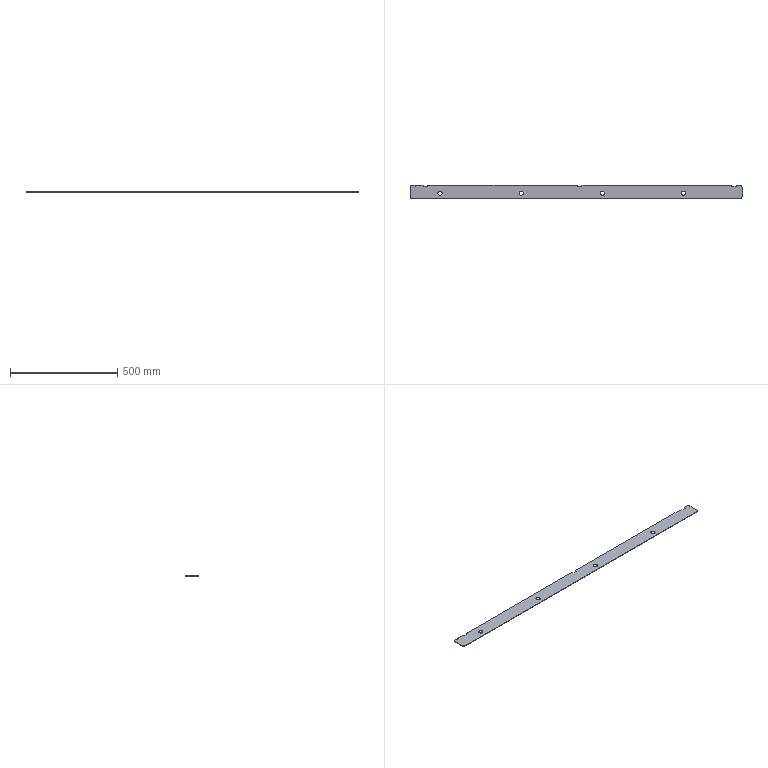Part | SolidWorks | features FlatPattern 1, SMBaseFlange 1, SheetMetal 1 | 1 solid | 34 faces | box 1550 x 65 x 2.3 mm | volume 227708 mm3 | plane 22 | cylinder 12 | commonest cylinder face diameters 20 x12
STEP:
#1=CARTESIAN_POINT('',(1294.,-523.,2.3));
#2=VERTEX_POINT('',#1);
#3=CARTESIAN_POINT('',(1314.,-523.,2.3));
#4=VERTEX_POINT('',#3);
#5=CARTESIAN_POINT('',(1304.,-523.,2.3));
#6=DIRECTION('',(0.,0.,1.));
#7=DIRECTION('',(1.,0.,0.));
#8=AXIS2_PLACEMENT_3D('',#5,#6,#7);
#9=CIRCLE('',#8,10.);
#10=EDGE_CURVE('',#2,#4,#9,.T.);
#11=ORIENTED_EDGE('',*,*,#10,.T.);
#12=CARTESIAN_POINT('',(1314.,-523.,0.));
#13=VERTEX_POINT('',#12);
#14=CARTESIAN_POINT('',(1314.,-523.,2.3));
#15=DIRECTION('',(0.,0.,-1.));
#16=VECTOR('',#15,1000.);
#17=LINE('',#14,#16);
#18=EDGE_CURVE('',#4,#13,#17,.T.);
#19=ORIENTED_EDGE('',*,*,#18,.T.);
#20=CARTESIAN_POINT('',(1294.,-523.,0.));
#21=VERTEX_POINT('',#20);
#22=CARTESIAN_POINT('',(1304.,-523.,0.));
#23=DIRECTION('',(0.,0.,1.));
#24=DIRECTION('',(1.,0.,0.));
#25=AXIS2_PLACEMENT_3D('',#22,#23,#24);
#26=CIRCLE('',#25,10.);
#27=EDGE_CURVE('',#21,#13,#26,.T.);
#28=ORIENTED_EDGE('',*,*,#27,.F.);
#29=CARTESIAN_POINT('',(1294.,-523.,2.3));
#30=DIRECTION('',(0.,0.,-1.));
#31=VECTOR('',#30,1000.);
#32=LINE('',#29,#31);
#33=EDGE_CURVE('',#2,#21,#32,.T.);
#34=ORIENTED_EDGE('',*,*,#33,.F.);
#35=EDGE_LOOP('',(#11,#19,#28,#34));
#36=FACE_OUTER_BOUND('',#35,.T.);
#37=CARTESIAN_POINT('',(1304.,-523.,2.3));
#38=DIRECTION('',(0.,0.,-1.));
#39=DIRECTION('',(-1.,0.,0.));
#40=AXIS2_PLACEMENT_3D('',#37,#38,#39);
#41=CYLINDRICAL_SURFACE('',#40,10.);
#42=ADVANCED_FACE('',(#36),#41,.F.);
#43=CARTESIAN_POINT('',(915.,-523.,2.3));
#44=VERTEX_POINT('',#43);
#45=CARTESIAN_POINT('',(935.,-523.,2.3));
#46=VERTEX_POINT('',#45);
#47=CARTESIAN_POINT('',(925.,-523.,2.3));
#48=DIRECTION('',(0.,0.,1.));
#49=DIRECTION('',(1.,0.,0.));
#50=AXIS2_PLACEMENT_3D('',#47,#48,#49);
#51=CIRCLE('',#50,10.);
#52=EDGE_CURVE('',#44,#46,#51,.T.);
#53=ORIENTED_EDGE('',*,*,#52,.T.);
#54=CARTESIAN_POINT('',(935.,-523.,0.));
#55=VERTEX_POINT('',#54);
#56=CARTESIAN_POINT('',(935.,-523.,2.3));
#57=DIRECTION('',(0.,0.,-1.));
#58=VECTOR('',#57,1000.);
#59=LINE('',#56,#58);
#60=EDGE_CURVE('',#46,#55,#59,.T.);
#61=ORIENTED_EDGE('',*,*,#60,.T.);
#62=CARTESIAN_POINT('',(915.,-523.,0.));
#63=VERTEX_POINT('',#62);
#64=CARTESIAN_POINT('',(925.,-523.,0.));
#65=DIRECTION('',(0.,0.,1.));
#66=DIRECTION('',(1.,0.,0.));
#67=AXIS2_PLACEMENT_3D('',#64,#65,#66);
#68=CIRCLE('',#67,10.);
#69=EDGE_CURVE('',#63,#55,#68,.T.);
#70=ORIENTED_EDGE('',*,*,#69,.F.);
#71=CARTESIAN_POINT('',(915.,-523.,2.3));
#72=DIRECTION('',(0.,0.,-1.));
#73=VECTOR('',#72,1000.);
#74=LINE('',#71,#73);
#75=EDGE_CURVE('',#44,#63,#74,.T.);
#76=ORIENTED_EDGE('',*,*,#75,.F.);
#77=EDGE_LOOP('',(#53,#61,#70,#76));
#78=FACE_OUTER_BOUND('',#77,.T.);
#79=CARTESIAN_POINT('',(925.,-523.,2.3));
#80=DIRECTION('',(0.,0.,-1.));
#81=DIRECTION('',(-1.,0.,0.));
#82=AXIS2_PLACEMENT_3D('',#79,#80,#81);
#83=CYLINDRICAL_SURFACE('',#82,10.);
#84=ADVANCED_FACE('',(#78),#83,.F.);
#85=CARTESIAN_POINT('',(536.,-523.,2.3));
#86=VERTEX_POINT('',#85);
#87=CARTESIAN_POINT('',(556.,-523.,2.3));
#88=VERTEX_POINT('',#87);
#89=CARTESIAN_POINT('',(546.,-523.,2.3));
#90=DIRECTION('',(0.,0.,1.));
#91=DIRECTION('',(1.,0.,0.));
#92=AXIS2_PLACEMENT_3D('',#89,#90,#91);
#93=CIRCLE('',#92,10.);
#94=EDGE_CURVE('',#86,#88,#93,.T.);
#95=ORIENTED_EDGE('',*,*,#94,.T.);
#96=CARTESIAN_POINT('',(556.,-523.,0.));
#97=VERTEX_POINT('',#96);
#98=CARTESIAN_POINT('',(556.,-523.,2.3));
#99=DIRECTION('',(0.,0.,-1.));
#100=VECTOR('',#99,1000.);
#101=LINE('',#98,#100);
#102=EDGE_CURVE('',#88,#97,#101,.T.);
#103=ORIENTED_EDGE('',*,*,#102,.T.);
#104=CARTESIAN_POINT('',(536.,-523.,0.));
#105=VERTEX_POINT('',#104);
#106=CARTESIAN_POINT('',(546.,-523.,0.));
#107=DIRECTION('',(0.,0.,1.));
#108=DIRECTION('',(1.,0.,0.));
#109=AXIS2_PLACEMENT_3D('',#106,#107,#108);
#110=CIRCLE('',#109,10.);
#111=EDGE_CURVE('',#105,#97,#110,.T.);
#112=ORIENTED_EDGE('',*,*,#111,.F.);
#113=CARTESIAN_POINT('',(536.,-523.,2.3));
#114=DIRECTION('',(0.,0.,-1.));
#115=VECTOR('',#114,1000.);
#116=LINE('',#113,#115);
#117=EDGE_CURVE('',#86,#105,#116,.T.);
#118=ORIENTED_EDGE('',*,*,#117,.F.);
#119=EDGE_LOOP('',(#95,#103,#112,#118));
#120=FACE_OUTER_BOUND('',#119,.T.);
#121=CARTESIAN_POINT('',(546.,-523.,2.3));
#122=DIRECTION('',(0.,0.,-1.));
#123=DIRECTION('',(-1.,0.,0.));
#124=AXIS2_PLACEMENT_3D('',#121,#122,#123);
#125=CYLINDRICAL_SURFACE('',#124,10.);
#126=ADVANCED_FACE('',(#120),#125,.F.);
#127=CARTESIAN_POINT('',(157.,-523.,2.3));
#128=VERTEX_POINT('',#127);
#129=CARTESIAN_POINT('',(177.,-523.,2.3));
#130=VERTEX_POINT('',#129);
#131=CARTESIAN_POINT('',(167.,-523.,2.3));
#132=DIRECTION('',(0.,0.,1.));
#133=DIRECTION('',(1.,0.,0.));
#134=AXIS2_PLACEMENT_3D('',#131,#132,#133);
#135=CIRCLE('',#134,10.);
#136=EDGE_CURVE('',#128,#130,#135,.T.);
#137=ORIENTED_EDGE('',*,*,#136,.T.);
#138=CARTESIAN_POINT('',(177.,-523.,0.));
#139=VERTEX_POINT('',#138);
#140=CARTESIAN_POINT('',(177.,-523.,2.3));
#141=DIRECTION('',(0.,0.,-1.));
#142=VECTOR('',#141,1000.);
#143=LINE('',#140,#142);
#144=EDGE_CURVE('',#130,#139,#143,.T.);
#145=ORIENTED_EDGE('',*,*,#144,.T.);
#146=CARTESIAN_POINT('',(157.,-523.,0.));
#147=VERTEX_POINT('',#146);
#148=CARTESIAN_POINT('',(167.,-523.,0.));
#149=DIRECTION('',(0.,0.,1.));
#150=DIRECTION('',(1.,0.,0.));
#151=AXIS2_PLACEMENT_3D('',#148,#149,#150);
#152=CIRCLE('',#151,10.);
#153=EDGE_CURVE('',#147,#139,#152,.T.);
#154=ORIENTED_EDGE('',*,*,#153,.F.);
#155=CARTESIAN_POINT('',(157.,-523.,2.3));
#156=DIRECTION('',(0.,0.,-1.));
#157=VECTOR('',#156,1000.);
#158=LINE('',#155,#157);
#159=EDGE_CURVE('',#128,#147,#158,.T.);
#160=ORIENTED_EDGE('',*,*,#159,.F.);
#161=EDGE_LOOP('',(#137,#145,#154,#160));
#162=FACE_OUTER_BOUND('',#161,.T.);
#163=CARTESIAN_POINT('',(167.,-523.,2.3));
#164=DIRECTION('',(0.,0.,-1.));
#165=DIRECTION('',(-1.,0.,0.));
#166=AXIS2_PLACEMENT_3D('',#163,#164,#165);
#167=CYLINDRICAL_SURFACE('',#166,10.);
#168=ADVANCED_FACE('',(#162),#167,.F.);
#169=CARTESIAN_POINT('',(50.4,-485.,2.3));
#170=VERTEX_POINT('',#169);
#171=CARTESIAN_POINT('',(37.,-485.,2.3));
#172=VERTEX_POINT('',#171);
#173=CARTESIAN_POINT('',(50.4,-485.,2.3));
#174=DIRECTION('',(-1.,0.,0.));
#175=VECTOR('',#174,1000.);
#176=LINE('',#173,#175);
#177=EDGE_CURVE('',#170,#172,#176,.T.);
#178=ORIENTED_EDGE('',*,*,#177,.T.);
#179=CARTESIAN_POINT('',(27.,-495.,2.3));
#180=VERTEX_POINT('',#179);
#181=CARTESIAN_POINT('',(37.,-495.,2.3));
#182=DIRECTION('',(0.,0.,1.));
#183=DIRECTION('',(-1.,0.,0.));
#184=AXIS2_PLACEMENT_3D('',#181,#182,#183);
#185=CIRCLE('',#184,10.);
#186=EDGE_CURVE('',#172,#180,#185,.T.);
#187=ORIENTED_EDGE('',*,*,#186,.T.);
#188=CARTESIAN_POINT('',(27.,-540.,2.3));
#189=VERTEX_POINT('',#188);
#190=CARTESIAN_POINT('',(27.,-540.,2.3));
#191=DIRECTION('',(0.,-1.,0.));
#192=VECTOR('',#191,1000.);
#193=LINE('',#190,#192);
#194=EDGE_CURVE('',#180,#189,#193,.T.);
#195=ORIENTED_EDGE('',*,*,#194,.T.);
#196=CARTESIAN_POINT('',(37.,-550.,2.3));
#197=VERTEX_POINT('',#196);
#198=CARTESIAN_POINT('',(37.,-540.,2.3));
#199=DIRECTION('',(0.,0.,1.));
#200=DIRECTION('',(-1.,0.,0.));
#201=AXIS2_PLACEMENT_3D('',#198,#199,#200);
#202=CIRCLE('',#201,10.);
#203=EDGE_CURVE('',#189,#197,#202,.T.);
#204=ORIENTED_EDGE('',*,*,#203,.T.);
#205=CARTESIAN_POINT('',(1567.,-550.,2.3));
#206=VERTEX_POINT('',#205);
#207=CARTESIAN_POINT('',(37.,-550.,2.3));
#208=DIRECTION('',(1.,0.,0.));
#209=VECTOR('',#208,1000.);
#210=LINE('',#207,#209);
#211=EDGE_CURVE('',#197,#206,#210,.T.);
#212=ORIENTED_EDGE('',*,*,#211,.T.);
#213=CARTESIAN_POINT('',(1577.,-540.,2.3));
#214=VERTEX_POINT('',#213);
#215=CARTESIAN_POINT('',(1567.,-540.,2.3));
#216=DIRECTION('',(0.,0.,1.));
#217=DIRECTION('',(1.,0.,0.));
#218=AXIS2_PLACEMENT_3D('',#215,#216,#217);
#219=CIRCLE('',#218,10.);
#220=EDGE_CURVE('',#206,#214,#219,.T.);
#221=ORIENTED_EDGE('',*,*,#220,.T.);
#222=CARTESIAN_POINT('',(1577.,-495.,2.3));
#223=VERTEX_POINT('',#222);
#224=CARTESIAN_POINT('',(1577.,-540.,2.3));
#225=DIRECTION('',(0.,1.,0.));
#226=VECTOR('',#225,1000.);
#227=LINE('',#224,#226);
#228=EDGE_CURVE('',#214,#223,#227,.T.);
#229=ORIENTED_EDGE('',*,*,#228,.T.);
#230=CARTESIAN_POINT('',(1567.,-485.,2.3));
#231=VERTEX_POINT('',#230);
#232=CARTESIAN_POINT('',(1567.,-495.,2.3));
#233=DIRECTION('',(0.,0.,1.));
#234=DIRECTION('',(1.,0.,0.));
#235=AXIS2_PLACEMENT_3D('',#232,#233,#234);
#236=CIRCLE('',#235,10.);
#237=EDGE_CURVE('',#223,#231,#236,.T.);
#238=ORIENTED_EDGE('',*,*,#237,.T.);
#239=CARTESIAN_POINT('',(1550.,-485.,2.3));
#240=VERTEX_POINT('',#239);
#241=CARTESIAN_POINT('',(1567.,-485.,2.3));
#242=DIRECTION('',(-1.,0.,0.));
#243=VECTOR('',#242,1000.);
#244=LINE('',#241,#243);
#245=EDGE_CURVE('',#231,#240,#244,.T.);
#246=ORIENTED_EDGE('',*,*,#245,.T.);
#247=CARTESIAN_POINT('',(1550.,-491.,2.3));
#248=VERTEX_POINT('',#247);
#249=CARTESIAN_POINT('',(1550.,-485.,2.3));
#250=DIRECTION('',(0.,-1.,0.));
#251=VECTOR('',#250,1000.);
#252=LINE('',#249,#251);
#253=EDGE_CURVE('',#240,#248,#252,.T.);
#254=ORIENTED_EDGE('',*,*,#253,.T.);
#255=CARTESIAN_POINT('',(1528.,-491.,2.3));
#256=VERTEX_POINT('',#255);
#257=CARTESIAN_POINT('',(1550.,-491.,2.3));
#258=DIRECTION('',(-1.,0.,0.));
#259=VECTOR('',#258,1000.);
#260=LINE('',#257,#259);
#261=EDGE_CURVE('',#248,#256,#260,.T.);
#262=ORIENTED_EDGE('',*,*,#261,.T.);
#263=CARTESIAN_POINT('',(1528.,-485.,2.3));
#264=VERTEX_POINT('',#263);
#265=CARTESIAN_POINT('',(1528.,-491.,2.3));
#266=DIRECTION('',(0.,1.,0.));
#267=VECTOR('',#266,1000.);
#268=LINE('',#265,#267);
#269=EDGE_CURVE('',#256,#264,#268,.T.);
#270=ORIENTED_EDGE('',*,*,#269,.T.);
#271=CARTESIAN_POINT('',(830.,-485.,2.3));
#272=VERTEX_POINT('',#271);
#273=CARTESIAN_POINT('',(1528.,-485.,2.3));
#274=DIRECTION('',(-1.,0.,0.));
#275=VECTOR('',#274,1000.);
#276=LINE('',#273,#275);
#277=EDGE_CURVE('',#264,#272,#276,.T.);
#278=ORIENTED_EDGE('',*,*,#277,.T.);
#279=CARTESIAN_POINT('',(830.,-491.,2.3));
#280=VERTEX_POINT('',#279);
#281=CARTESIAN_POINT('',(830.,-485.,2.3));
#282=DIRECTION('',(0.,-1.,0.));
#283=VECTOR('',#282,1000.);
#284=LINE('',#281,#283);
#285=EDGE_CURVE('',#272,#280,#284,.T.);
#286=ORIENTED_EDGE('',*,*,#285,.T.);
#287=CARTESIAN_POINT('',(808.,-491.,2.3));
#288=VERTEX_POINT('',#287);
#289=CARTESIAN_POINT('',(830.,-491.,2.3));
#290=DIRECTION('',(-1.,0.,0.));
#291=VECTOR('',#290,1000.);
#292=LINE('',#289,#291);
#293=EDGE_CURVE('',#280,#288,#292,.T.);
#294=ORIENTED_EDGE('',*,*,#293,.T.);
#295=CARTESIAN_POINT('',(808.,-485.,2.3));
#296=VERTEX_POINT('',#295);
#297=CARTESIAN_POINT('',(808.,-491.,2.3));
#298=DIRECTION('',(0.,1.,0.));
#299=VECTOR('',#298,1000.);
#300=LINE('',#297,#299);
#301=EDGE_CURVE('',#288,#296,#300,.T.);
#302=ORIENTED_EDGE('',*,*,#301,.T.);
#303=CARTESIAN_POINT('',(110.,-485.,2.3));
#304=VERTEX_POINT('',#303);
#305=CARTESIAN_POINT('',(808.,-485.,2.3));
#306=DIRECTION('',(-1.,0.,0.));
#307=VECTOR('',#306,1000.);
#308=LINE('',#305,#307);
#309=EDGE_CURVE('',#296,#304,#308,.T.);
#310=ORIENTED_EDGE('',*,*,#309,.T.);
#311=CARTESIAN_POINT('',(110.,-491.,2.3));
#312=VERTEX_POINT('',#311);
#313=CARTESIAN_POINT('',(110.,-485.,2.3));
#314=DIRECTION('',(0.,-1.,0.));
#315=VECTOR('',#314,1000.);
#316=LINE('',#313,#315);
#317=EDGE_CURVE('',#304,#312,#316,.T.);
#318=ORIENTED_EDGE('',*,*,#317,.T.);
#319=CARTESIAN_POINT('',(88.,-491.,2.3));
#320=VERTEX_POINT('',#319);
#321=CARTESIAN_POINT('',(110.,-491.,2.3));
#322=DIRECTION('',(-1.,0.,0.));
#323=VECTOR('',#322,1000.);
#324=LINE('',#321,#323);
#325=EDGE_CURVE('',#312,#320,#324,.T.);
#326=ORIENTED_EDGE('',*,*,#325,.T.);
#327=CARTESIAN_POINT('',(88.,-485.,2.3));
#328=VERTEX_POINT('',#327);
#329=CARTESIAN_POINT('',(88.,-491.,2.3));
#330=DIRECTION('',(0.,1.,0.));
#331=VECTOR('',#330,1000.);
#332=LINE('',#329,#331);
#333=EDGE_CURVE('',#320,#328,#332,.T.);
#334=ORIENTED_EDGE('',*,*,#333,.T.);
#335=CARTESIAN_POINT('',(52.,-485.,2.3));
#336=VERTEX_POINT('',#335);
#337=CARTESIAN_POINT('',(88.,-485.,2.3));
#338=DIRECTION('',(-1.,0.,0.));
#339=VECTOR('',#338,1000.);
#340=LINE('',#337,#339);
#341=EDGE_CURVE('',#328,#336,#340,.T.);
#342=ORIENTED_EDGE('',*,*,#341,.T.);
#343=CARTESIAN_POINT('',(52.,-490.,2.3));
#344=VERTEX_POINT('',#343);
#345=CARTESIAN_POINT('',(52.,-490.,2.3));
#346=DIRECTION('',(0.,-1.,0.));
#347=VECTOR('',#346,1000.);
#348=LINE('',#345,#347);
#349=EDGE_CURVE('',#336,#344,#348,.T.);
#350=ORIENTED_EDGE('',*,*,#349,.T.);
#351=CARTESIAN_POINT('',(50.4,-490.,2.3));
#352=VERTEX_POINT('',#351);
#353=CARTESIAN_POINT('',(52.,-490.,2.3));
#354=DIRECTION('',(-1.,0.,0.));
#355=VECTOR('',#354,1000.);
#356=LINE('',#353,#355);
#357=EDGE_CURVE('',#344,#352,#356,.T.);
#358=ORIENTED_EDGE('',*,*,#357,.T.);
#359=CARTESIAN_POINT('',(50.4,-490.,2.3));
#360=DIRECTION('',(0.,1.,0.));
#361=VECTOR('',#360,1000.);
#362=LINE('',#359,#361);
#363=EDGE_CURVE('',#352,#170,#362,.T.);
#364=ORIENTED_EDGE('',*,*,#363,.T.);
#365=EDGE_LOOP('',(#178,#187,#195,#204,#212,#221,#229,#238,#246,#254,#262,#270,#278,#286,#294,#302,#310,#318,#326,#334,#342,#350,#358,#364));
#366=FACE_OUTER_BOUND('',#365,.T.);
#367=ORIENTED_EDGE('',*,*,#136,.F.);
#368=CARTESIAN_POINT('',(167.,-523.,2.3));
#369=DIRECTION('',(0.,0.,1.));
#370=DIRECTION('',(1.,0.,0.));
#371=AXIS2_PLACEMENT_3D('',#368,#369,#370);
#372=CIRCLE('',#371,10.);
#373=EDGE_CURVE('',#130,#128,#372,.T.);
#374=ORIENTED_EDGE('',*,*,#373,.F.);
#375=EDGE_LOOP('',(#367,#374));
#376=FACE_BOUND('',#375,.T.);
#377=ORIENTED_EDGE('',*,*,#94,.F.);
#378=CARTESIAN_POINT('',(546.,-523.,2.3));
#379=DIRECTION('',(0.,0.,1.));
#380=DIRECTION('',(1.,0.,0.));
#381=AXIS2_PLACEMENT_3D('',#378,#379,#380);
#382=CIRCLE('',#381,10.);
#383=EDGE_CURVE('',#88,#86,#382,.T.);
#384=ORIENTED_EDGE('',*,*,#383,.F.);
#385=EDGE_LOOP('',(#377,#384));
#386=FACE_BOUND('',#385,.T.);
#387=ORIENTED_EDGE('',*,*,#52,.F.);
#388=CARTESIAN_POINT('',(925.,-523.,2.3));
#389=DIRECTION('',(0.,0.,1.));
#390=DIRECTION('',(1.,0.,0.));
#391=AXIS2_PLACEMENT_3D('',#388,#389,#390);
#392=CIRCLE('',#391,10.);
#393=EDGE_CURVE('',#46,#44,#392,.T.);
#394=ORIENTED_EDGE('',*,*,#393,.F.);
#395=EDGE_LOOP('',(#387,#394));
#396=FACE_BOUND('',#395,.T.);
#397=ORIENTED_EDGE('',*,*,#10,.F.);
#398=CARTESIAN_POINT('',(1304.,-523.,2.3));
#399=DIRECTION('',(0.,0.,1.));
#400=DIRECTION('',(1.,0.,0.));
#401=AXIS2_PLACEMENT_3D('',#398,#399,#400);
#402=CIRCLE('',#401,10.);
#403=EDGE_CURVE('',#4,#2,#402,.T.);
#404=ORIENTED_EDGE('',*,*,#403,.F.);
#405=EDGE_LOOP('',(#397,#404));
#406=FACE_BOUND('',#405,.T.);
#407=CARTESIAN_POINT('',(37.,-495.,2.3));
#408=DIRECTION('',(0.,0.,-1.));
#409=DIRECTION('',(-1.,0.,0.));
#410=AXIS2_PLACEMENT_3D('',#407,#408,#409);
#411=PLANE('',#410);
#412=ADVANCED_FACE('',(#366,#376,#386,#396,#406),#411,.F.);
#413=ORIENTED_EDGE('',*,*,#69,.T.);
#414=CARTESIAN_POINT('',(925.,-523.,0.));
#415=DIRECTION('',(0.,0.,1.));
#416=DIRECTION('',(1.,0.,0.));
#417=AXIS2_PLACEMENT_3D('',#414,#415,#416);
#418=CIRCLE('',#417,10.);
#419=EDGE_CURVE('',#55,#63,#418,.T.);
#420=ORIENTED_EDGE('',*,*,#419,.T.);
#421=EDGE_LOOP('',(#413,#420));
#422=FACE_BOUND('',#421,.T.);
#423=ORIENTED_EDGE('',*,*,#153,.T.);
#424=CARTESIAN_POINT('',(167.,-523.,0.));
#425=DIRECTION('',(0.,0.,1.));
#426=DIRECTION('',(1.,0.,0.));
#427=AXIS2_PLACEMENT_3D('',#424,#425,#426);
#428=CIRCLE('',#427,10.);
#429=EDGE_CURVE('',#139,#147,#428,.T.);
#430=ORIENTED_EDGE('',*,*,#429,.T.);
#431=EDGE_LOOP('',(#423,#430));
#432=FACE_BOUND('',#431,.T.);
#433=CARTESIAN_POINT('',(50.4,-485.,0.));
#434=VERTEX_POINT('',#433);
#435=CARTESIAN_POINT('',(37.,-485.,0.));
#436=VERTEX_POINT('',#435);
#437=CARTESIAN_POINT('',(50.4,-485.,0.));
#438=DIRECTION('',(-1.,0.,0.));
#439=VECTOR('',#438,1000.);
#440=LINE('',#437,#439);
#441=EDGE_CURVE('',#434,#436,#440,.T.);
#442=ORIENTED_EDGE('',*,*,#441,.F.);
#443=CARTESIAN_POINT('',(50.4,-490.,0.));
#444=VERTEX_POINT('',#443);
#445=CARTESIAN_POINT('',(50.4,-490.,0.));
#446=DIRECTION('',(0.,1.,0.));
#447=VECTOR('',#446,1000.);
#448=LINE('',#445,#447);
#449=EDGE_CURVE('',#444,#434,#448,.T.);
#450=ORIENTED_EDGE('',*,*,#449,.F.);
#451=CARTESIAN_POINT('',(52.,-490.,0.));
#452=VERTEX_POINT('',#451);
#453=CARTESIAN_POINT('',(52.,-490.,0.));
#454=DIRECTION('',(-1.,0.,0.));
#455=VECTOR('',#454,1000.);
#456=LINE('',#453,#455);
#457=EDGE_CURVE('',#452,#444,#456,.T.);
#458=ORIENTED_EDGE('',*,*,#457,.F.);
#459=CARTESIAN_POINT('',(52.,-485.,0.));
#460=VERTEX_POINT('',#459);
#461=CARTESIAN_POINT('',(52.,-490.,0.));
#462=DIRECTION('',(0.,-1.,0.));
#463=VECTOR('',#462,1000.);
#464=LINE('',#461,#463);
#465=EDGE_CURVE('',#460,#452,#464,.T.);
#466=ORIENTED_EDGE('',*,*,#465,.F.);
#467=CARTESIAN_POINT('',(88.,-485.,0.));
#468=VERTEX_POINT('',#467);
#469=CARTESIAN_POINT('',(88.,-485.,0.));
#470=DIRECTION('',(-1.,0.,0.));
#471=VECTOR('',#470,1000.);
#472=LINE('',#469,#471);
#473=EDGE_CURVE('',#468,#460,#472,.T.);
#474=ORIENTED_EDGE('',*,*,#473,.F.);
#475=CARTESIAN_POINT('',(88.,-491.,0.));
#476=VERTEX_POINT('',#475);
#477=CARTESIAN_POINT('',(88.,-491.,0.));
#478=DIRECTION('',(0.,1.,0.));
#479=VECTOR('',#478,1000.);
#480=LINE('',#477,#479);
#481=EDGE_CURVE('',#476,#468,#480,.T.);
#482=ORIENTED_EDGE('',*,*,#481,.F.);
#483=CARTESIAN_POINT('',(110.,-491.,0.));
#484=VERTEX_POINT('',#483);
#485=CARTESIAN_POINT('',(110.,-491.,0.));
#486=DIRECTION('',(-1.,0.,0.));
#487=VECTOR('',#486,1000.);
#488=LINE('',#485,#487);
#489=EDGE_CURVE('',#484,#476,#488,.T.);
#490=ORIENTED_EDGE('',*,*,#489,.F.);
#491=CARTESIAN_POINT('',(110.,-485.,0.));
#492=VERTEX_POINT('',#491);
#493=CARTESIAN_POINT('',(110.,-485.,0.));
#494=DIRECTION('',(0.,-1.,0.));
#495=VECTOR('',#494,1000.);
#496=LINE('',#493,#495);
#497=EDGE_CURVE('',#492,#484,#496,.T.);
#498=ORIENTED_EDGE('',*,*,#497,.F.);
#499=CARTESIAN_POINT('',(808.,-485.,0.));
#500=VERTEX_POINT('',#499);
#501=CARTESIAN_POINT('',(808.,-485.,0.));
#502=DIRECTION('',(-1.,0.,0.));
#503=VECTOR('',#502,1000.);
#504=LINE('',#501,#503);
#505=EDGE_CURVE('',#500,#492,#504,.T.);
#506=ORIENTED_EDGE('',*,*,#505,.F.);
#507=CARTESIAN_POINT('',(808.,-491.,0.));
#508=VERTEX_POINT('',#507);
#509=CARTESIAN_POINT('',(808.,-491.,0.));
#510=DIRECTION('',(0.,1.,0.));
#511=VECTOR('',#510,1000.);
#512=LINE('',#509,#511);
#513=EDGE_CURVE('',#508,#500,#512,.T.);
#514=ORIENTED_EDGE('',*,*,#513,.F.);
#515=CARTESIAN_POINT('',(830.,-491.,0.));
#516=VERTEX_POINT('',#515);
#517=CARTESIAN_POINT('',(830.,-491.,0.));
#518=DIRECTION('',(-1.,0.,0.));
#519=VECTOR('',#518,1000.);
#520=LINE('',#517,#519);
#521=EDGE_CURVE('',#516,#508,#520,.T.);
#522=ORIENTED_EDGE('',*,*,#521,.F.);
#523=CARTESIAN_POINT('',(830.,-485.,0.));
#524=VERTEX_POINT('',#523);
#525=CARTESIAN_POINT('',(830.,-485.,0.));
#526=DIRECTION('',(0.,-1.,0.));
#527=VECTOR('',#526,1000.);
#528=LINE('',#525,#527);
#529=EDGE_CURVE('',#524,#516,#528,.T.);
#530=ORIENTED_EDGE('',*,*,#529,.F.);
#531=CARTESIAN_POINT('',(1528.,-485.,0.));
#532=VERTEX_POINT('',#531);
#533=CARTESIAN_POINT('',(1528.,-485.,0.));
#534=DIRECTION('',(-1.,0.,0.));
#535=VECTOR('',#534,1000.);
#536=LINE('',#533,#535);
#537=EDGE_CURVE('',#532,#524,#536,.T.);
#538=ORIENTED_EDGE('',*,*,#537,.F.);
#539=CARTESIAN_POINT('',(1528.,-491.,0.));
#540=VERTEX_POINT('',#539);
#541=CARTESIAN_POINT('',(1528.,-491.,0.));
#542=DIRECTION('',(0.,1.,0.));
#543=VECTOR('',#542,1000.);
#544=LINE('',#541,#543);
#545=EDGE_CURVE('',#540,#532,#544,.T.);
#546=ORIENTED_EDGE('',*,*,#545,.F.);
#547=CARTESIAN_POINT('',(1550.,-491.,0.));
#548=VERTEX_POINT('',#547);
#549=CARTESIAN_POINT('',(1550.,-491.,0.));
#550=DIRECTION('',(-1.,0.,0.));
#551=VECTOR('',#550,1000.);
#552=LINE('',#549,#551);
#553=EDGE_CURVE('',#548,#540,#552,.T.);
#554=ORIENTED_EDGE('',*,*,#553,.F.);
#555=CARTESIAN_POINT('',(1550.,-485.,0.));
#556=VERTEX_POINT('',#555);
#557=CARTESIAN_POINT('',(1550.,-485.,0.));
#558=DIRECTION('',(0.,-1.,0.));
#559=VECTOR('',#558,1000.);
#560=LINE('',#557,#559);
#561=EDGE_CURVE('',#556,#548,#560,.T.);
#562=ORIENTED_EDGE('',*,*,#561,.F.);
#563=CARTESIAN_POINT('',(1567.,-485.,0.));
#564=VERTEX_POINT('',#563);
#565=CARTESIAN_POINT('',(1567.,-485.,0.));
#566=DIRECTION('',(-1.,0.,0.));
#567=VECTOR('',#566,1000.);
#568=LINE('',#565,#567);
#569=EDGE_CURVE('',#564,#556,#568,.T.);
#570=ORIENTED_EDGE('',*,*,#569,.F.);
#571=CARTESIAN_POINT('',(1577.,-495.,0.));
#572=VERTEX_POINT('',#571);
#573=CARTESIAN_POINT('',(1567.,-495.,0.));
#574=DIRECTION('',(0.,0.,1.));
#575=DIRECTION('',(1.,0.,0.));
#576=AXIS2_PLACEMENT_3D('',#573,#574,#575);
#577=CIRCLE('',#576,10.);
#578=EDGE_CURVE('',#572,#564,#577,.T.);
#579=ORIENTED_EDGE('',*,*,#578,.F.);
#580=CARTESIAN_POINT('',(1577.,-540.,0.));
#581=VERTEX_POINT('',#580);
#582=CARTESIAN_POINT('',(1577.,-540.,0.));
#583=DIRECTION('',(0.,1.,0.));
#584=VECTOR('',#583,1000.);
#585=LINE('',#582,#584);
#586=EDGE_CURVE('',#581,#572,#585,.T.);
#587=ORIENTED_EDGE('',*,*,#586,.F.);
#588=CARTESIAN_POINT('',(1567.,-550.,0.));
#589=VERTEX_POINT('',#588);
#590=CARTESIAN_POINT('',(1567.,-540.,0.));
#591=DIRECTION('',(0.,0.,1.));
#592=DIRECTION('',(1.,0.,0.));
#593=AXIS2_PLACEMENT_3D('',#590,#591,#592);
#594=CIRCLE('',#593,10.);
#595=EDGE_CURVE('',#589,#581,#594,.T.);
#596=ORIENTED_EDGE('',*,*,#595,.F.);
#597=CARTESIAN_POINT('',(37.,-550.,0.));
#598=VERTEX_POINT('',#597);
#599=CARTESIAN_POINT('',(37.,-550.,0.));
#600=DIRECTION('',(1.,0.,0.));
#601=VECTOR('',#600,1000.);
#602=LINE('',#599,#601);
#603=EDGE_CURVE('',#598,#589,#602,.T.);
#604=ORIENTED_EDGE('',*,*,#603,.F.);
#605=CARTESIAN_POINT('',(27.,-540.,0.));
#606=VERTEX_POINT('',#605);
#607=CARTESIAN_POINT('',(37.,-540.,0.));
#608=DIRECTION('',(0.,0.,1.));
#609=DIRECTION('',(-1.,0.,0.));
#610=AXIS2_PLACEMENT_3D('',#607,#608,#609);
#611=CIRCLE('',#610,10.);
#612=EDGE_CURVE('',#606,#598,#611,.T.);
#613=ORIENTED_EDGE('',*,*,#612,.F.);
#614=CARTESIAN_POINT('',(27.,-495.,0.));
#615=VERTEX_POINT('',#614);
#616=CARTESIAN_POINT('',(27.,-540.,0.));
#617=DIRECTION('',(0.,-1.,0.));
#618=VECTOR('',#617,1000.);
#619=LINE('',#616,#618);
#620=EDGE_CURVE('',#615,#606,#619,.T.);
#621=ORIENTED_EDGE('',*,*,#620,.F.);
#622=CARTESIAN_POINT('',(37.,-495.,0.));
#623=DIRECTION('',(0.,0.,1.));
#624=DIRECTION('',(-1.,0.,0.));
#625=AXIS2_PLACEMENT_3D('',#622,#623,#624);
#626=CIRCLE('',#625,10.);
#627=EDGE_CURVE('',#436,#615,#626,.T.);
#628=ORIENTED_EDGE('',*,*,#627,.F.);
#629=EDGE_LOOP('',(#442,#450,#458,#466,#474,#482,#490,#498,#506,#514,#522,#530,#538,#546,#554,#562,#570,#579,#587,#596,#604,#613,#621,#628));
#630=FACE_OUTER_BOUND('',#629,.T.);
#631=ORIENTED_EDGE('',*,*,#111,.T.);
#632=CARTESIAN_POINT('',(546.,-523.,0.));
#633=DIRECTION('',(0.,0.,1.));
#634=DIRECTION('',(1.,0.,0.));
#635=AXIS2_PLACEMENT_3D('',#632,#633,#634);
#636=CIRCLE('',#635,10.);
#637=EDGE_CURVE('',#97,#105,#636,.T.);
#638=ORIENTED_EDGE('',*,*,#637,.T.);
#639=EDGE_LOOP('',(#631,#638));
#640=FACE_BOUND('',#639,.T.);
#641=ORIENTED_EDGE('',*,*,#27,.T.);
#642=CARTESIAN_POINT('',(1304.,-523.,0.));
#643=DIRECTION('',(0.,0.,1.));
#644=DIRECTION('',(1.,0.,0.));
#645=AXIS2_PLACEMENT_3D('',#642,#643,#644);
#646=CIRCLE('',#645,10.);
#647=EDGE_CURVE('',#13,#21,#646,.T.);
#648=ORIENTED_EDGE('',*,*,#647,.T.);
#649=EDGE_LOOP('',(#641,#648));
#650=FACE_BOUND('',#649,.T.);
#651=CARTESIAN_POINT('',(37.,-495.,0.));
#652=DIRECTION('',(0.,0.,-1.));
#653=DIRECTION('',(-1.,0.,0.));
#654=AXIS2_PLACEMENT_3D('',#651,#652,#653);
#655=PLANE('',#654);
#656=ADVANCED_FACE('',(#422,#432,#630,#640,#650),#655,.T.);
#657=ORIENTED_EDGE('',*,*,#441,.T.);
#658=CARTESIAN_POINT('',(37.,-485.,2.3));
#659=DIRECTION('',(0.,0.,-1.));
#660=VECTOR('',#659,1000.);
#661=LINE('',#658,#660);
#662=EDGE_CURVE('',#172,#436,#661,.T.);
#663=ORIENTED_EDGE('',*,*,#662,.F.);
#664=ORIENTED_EDGE('',*,*,#177,.F.);
#665=CARTESIAN_POINT('',(50.4,-485.,2.3));
#666=DIRECTION('',(0.,0.,-1.));
#667=VECTOR('',#666,1000.);
#668=LINE('',#665,#667);
#669=EDGE_CURVE('',#170,#434,#668,.T.);
#670=ORIENTED_EDGE('',*,*,#669,.T.);
#671=EDGE_LOOP('',(#657,#663,#664,#670));
#672=FACE_OUTER_BOUND('',#671,.T.);
#673=CARTESIAN_POINT('',(50.4,-485.,2.3));
#674=DIRECTION('',(0.,-1.,0.));
#675=DIRECTION('',(0.,0.,-1.));
#676=AXIS2_PLACEMENT_3D('',#673,#674,#675);
#677=PLANE('',#676);
#678=ADVANCED_FACE('',(#672),#677,.F.);
#679=ORIENTED_EDGE('',*,*,#627,.T.);
#680=CARTESIAN_POINT('',(27.,-495.,2.3));
#681=DIRECTION('',(0.,0.,-1.));
#682=VECTOR('',#681,1000.);
#683=LINE('',#680,#682);
#684=EDGE_CURVE('',#180,#615,#683,.T.);
#685=ORIENTED_EDGE('',*,*,#684,.F.);
#686=ORIENTED_EDGE('',*,*,#186,.F.);
#687=ORIENTED_EDGE('',*,*,#662,.T.);
#688=EDGE_LOOP('',(#679,#685,#686,#687));
#689=FACE_OUTER_BOUND('',#688,.T.);
#690=CARTESIAN_POINT('',(37.,-495.,2.3));
#691=DIRECTION('',(0.,0.,-1.));
#692=DIRECTION('',(-1.,0.,0.));
#693=AXIS2_PLACEMENT_3D('',#690,#691,#692);
#694=CYLINDRICAL_SURFACE('',#693,10.);
#695=ADVANCED_FACE('',(#689),#694,.T.);
#696=ORIENTED_EDGE('',*,*,#620,.T.);
#697=CARTESIAN_POINT('',(27.,-540.,2.3));
#698=DIRECTION('',(0.,0.,-1.));
#699=VECTOR('',#698,1000.);
#700=LINE('',#697,#699);
#701=EDGE_CURVE('',#189,#606,#700,.T.);
#702=ORIENTED_EDGE('',*,*,#701,.F.);
#703=ORIENTED_EDGE('',*,*,#194,.F.);
#704=ORIENTED_EDGE('',*,*,#684,.T.);
#705=EDGE_LOOP('',(#696,#702,#703,#704));
#706=FACE_OUTER_BOUND('',#705,.T.);
#707=CARTESIAN_POINT('',(27.,-540.,2.3));
#708=DIRECTION('',(1.,0.,0.));
#709=DIRECTION('',(0.,0.,-1.));
#710=AXIS2_PLACEMENT_3D('',#707,#708,#709);
#711=PLANE('',#710);
#712=ADVANCED_FACE('',(#706),#711,.F.);
#713=ORIENTED_EDGE('',*,*,#612,.T.);
#714=CARTESIAN_POINT('',(37.,-550.,2.3));
#715=DIRECTION('',(0.,0.,-1.));
#716=VECTOR('',#715,1000.);
#717=LINE('',#714,#716);
#718=EDGE_CURVE('',#197,#598,#717,.T.);
#719=ORIENTED_EDGE('',*,*,#718,.F.);
#720=ORIENTED_EDGE('',*,*,#203,.F.);
#721=ORIENTED_EDGE('',*,*,#701,.T.);
#722=EDGE_LOOP('',(#713,#719,#720,#721));
#723=FACE_OUTER_BOUND('',#722,.T.);
#724=CARTESIAN_POINT('',(37.,-540.,2.3));
#725=DIRECTION('',(0.,0.,-1.));
#726=DIRECTION('',(-1.,0.,0.));
#727=AXIS2_PLACEMENT_3D('',#724,#725,#726);
#728=CYLINDRICAL_SURFACE('',#727,10.);
#729=ADVANCED_FACE('',(#723),#728,.T.);
#730=ORIENTED_EDGE('',*,*,#603,.T.);
#731=CARTESIAN_POINT('',(1567.,-550.,2.3));
#732=DIRECTION('',(0.,0.,-1.));
#733=VECTOR('',#732,1000.);
#734=LINE('',#731,#733);
#735=EDGE_CURVE('',#206,#589,#734,.T.);
#736=ORIENTED_EDGE('',*,*,#735,.F.);
#737=ORIENTED_EDGE('',*,*,#211,.F.);
#738=ORIENTED_EDGE('',*,*,#718,.T.);
#739=EDGE_LOOP('',(#730,#736,#737,#738));
#740=FACE_OUTER_BOUND('',#739,.T.);
#741=CARTESIAN_POINT('',(37.,-550.,2.3));
#742=DIRECTION('',(0.,1.,0.));
#743=DIRECTION('',(0.,0.,1.));
#744=AXIS2_PLACEMENT_3D('',#741,#742,#743);
#745=PLANE('',#744);
#746=ADVANCED_FACE('',(#740),#745,.F.);
#747=ORIENTED_EDGE('',*,*,#595,.T.);
#748=CARTESIAN_POINT('',(1577.,-540.,2.3));
#749=DIRECTION('',(0.,0.,-1.));
#750=VECTOR('',#749,1000.);
#751=LINE('',#748,#750);
#752=EDGE_CURVE('',#214,#581,#751,.T.);
#753=ORIENTED_EDGE('',*,*,#752,.F.);
#754=ORIENTED_EDGE('',*,*,#220,.F.);
#755=ORIENTED_EDGE('',*,*,#735,.T.);
#756=EDGE_LOOP('',(#747,#753,#754,#755));
#757=FACE_OUTER_BOUND('',#756,.T.);
#758=CARTESIAN_POINT('',(1567.,-540.,2.3));
#759=DIRECTION('',(0.,0.,-1.));
#760=DIRECTION('',(-1.,0.,0.));
#761=AXIS2_PLACEMENT_3D('',#758,#759,#760);
#762=CYLINDRICAL_SURFACE('',#761,10.);
#763=ADVANCED_FACE('',(#757),#762,.T.);
#764=ORIENTED_EDGE('',*,*,#586,.T.);
#765=CARTESIAN_POINT('',(1577.,-495.,2.3));
#766=DIRECTION('',(0.,0.,-1.));
#767=VECTOR('',#766,1000.);
#768=LINE('',#765,#767);
#769=EDGE_CURVE('',#223,#572,#768,.T.);
#770=ORIENTED_EDGE('',*,*,#769,.F.);
#771=ORIENTED_EDGE('',*,*,#228,.F.);
#772=ORIENTED_EDGE('',*,*,#752,.T.);
#773=EDGE_LOOP('',(#764,#770,#771,#772));
#774=FACE_OUTER_BOUND('',#773,.T.);
#775=CARTESIAN_POINT('',(1577.,-540.,2.3));
#776=DIRECTION('',(-1.,0.,0.));
#777=DIRECTION('',(0.,0.,1.));
#778=AXIS2_PLACEMENT_3D('',#775,#776,#777);
#779=PLANE('',#778);
#780=ADVANCED_FACE('',(#774),#779,.F.);
#781=ORIENTED_EDGE('',*,*,#578,.T.);
#782=CARTESIAN_POINT('',(1567.,-485.,2.3));
#783=DIRECTION('',(0.,0.,-1.));
#784=VECTOR('',#783,1000.);
#785=LINE('',#782,#784);
#786=EDGE_CURVE('',#231,#564,#785,.T.);
#787=ORIENTED_EDGE('',*,*,#786,.F.);
#788=ORIENTED_EDGE('',*,*,#237,.F.);
#789=ORIENTED_EDGE('',*,*,#769,.T.);
#790=EDGE_LOOP('',(#781,#787,#788,#789));
#791=FACE_OUTER_BOUND('',#790,.T.);
#792=CARTESIAN_POINT('',(1567.,-495.,2.3));
#793=DIRECTION('',(0.,0.,-1.));
#794=DIRECTION('',(-1.,0.,0.));
#795=AXIS2_PLACEMENT_3D('',#792,#793,#794);
#796=CYLINDRICAL_SURFACE('',#795,10.);
#797=ADVANCED_FACE('',(#791),#796,.T.);
#798=ORIENTED_EDGE('',*,*,#569,.T.);
#799=CARTESIAN_POINT('',(1550.,-485.,2.3));
#800=DIRECTION('',(0.,0.,-1.));
#801=VECTOR('',#800,1000.);
#802=LINE('',#799,#801);
#803=EDGE_CURVE('',#240,#556,#802,.T.);
#804=ORIENTED_EDGE('',*,*,#803,.F.);
#805=ORIENTED_EDGE('',*,*,#245,.F.);
#806=ORIENTED_EDGE('',*,*,#786,.T.);
#807=EDGE_LOOP('',(#798,#804,#805,#806));
#808=FACE_OUTER_BOUND('',#807,.T.);
#809=CARTESIAN_POINT('',(1567.,-485.,2.3));
#810=DIRECTION('',(0.,-1.,0.));
#811=DIRECTION('',(0.,0.,-1.));
#812=AXIS2_PLACEMENT_3D('',#809,#810,#811);
#813=PLANE('',#812);
#814=ADVANCED_FACE('',(#808),#813,.F.);
#815=ORIENTED_EDGE('',*,*,#561,.T.);
#816=CARTESIAN_POINT('',(1550.,-491.,2.3));
#817=DIRECTION('',(0.,0.,-1.));
#818=VECTOR('',#817,1000.);
#819=LINE('',#816,#818);
#820=EDGE_CURVE('',#248,#548,#819,.T.);
#821=ORIENTED_EDGE('',*,*,#820,.F.);
#822=ORIENTED_EDGE('',*,*,#253,.F.);
#823=ORIENTED_EDGE('',*,*,#803,.T.);
#824=EDGE_LOOP('',(#815,#821,#822,#823));
#825=FACE_OUTER_BOUND('',#824,.T.);
#826=CARTESIAN_POINT('',(1550.,-485.,2.3));
#827=DIRECTION('',(1.,0.,0.));
#828=DIRECTION('',(0.,0.,-1.));
#829=AXIS2_PLACEMENT_3D('',#826,#827,#828);
#830=PLANE('',#829);
#831=ADVANCED_FACE('',(#825),#830,.F.);
#832=ORIENTED_EDGE('',*,*,#553,.T.);
#833=CARTESIAN_POINT('',(1528.,-491.,2.3));
#834=DIRECTION('',(0.,0.,-1.));
#835=VECTOR('',#834,1000.);
#836=LINE('',#833,#835);
#837=EDGE_CURVE('',#256,#540,#836,.T.);
#838=ORIENTED_EDGE('',*,*,#837,.F.);
#839=ORIENTED_EDGE('',*,*,#261,.F.);
#840=ORIENTED_EDGE('',*,*,#820,.T.);
#841=EDGE_LOOP('',(#832,#838,#839,#840));
#842=FACE_OUTER_BOUND('',#841,.T.);
#843=CARTESIAN_POINT('',(1550.,-491.,2.3));
#844=DIRECTION('',(0.,-1.,0.));
#845=DIRECTION('',(0.,0.,-1.));
#846=AXIS2_PLACEMENT_3D('',#843,#844,#845);
#847=PLANE('',#846);
#848=ADVANCED_FACE('',(#842),#847,.F.);
#849=ORIENTED_EDGE('',*,*,#545,.T.);
#850=CARTESIAN_POINT('',(1528.,-485.,2.3));
#851=DIRECTION('',(0.,0.,-1.));
#852=VECTOR('',#851,1000.);
#853=LINE('',#850,#852);
#854=EDGE_CURVE('',#264,#532,#853,.T.);
#855=ORIENTED_EDGE('',*,*,#854,.F.);
#856=ORIENTED_EDGE('',*,*,#269,.F.);
#857=ORIENTED_EDGE('',*,*,#837,.T.);
#858=EDGE_LOOP('',(#849,#855,#856,#857));
#859=FACE_OUTER_BOUND('',#858,.T.);
#860=CARTESIAN_POINT('',(1528.,-491.,2.3));
#861=DIRECTION('',(-1.,0.,0.));
#862=DIRECTION('',(0.,0.,1.));
#863=AXIS2_PLACEMENT_3D('',#860,#861,#862);
#864=PLANE('',#863);
#865=ADVANCED_FACE('',(#859),#864,.F.);
#866=ORIENTED_EDGE('',*,*,#537,.T.);
#867=CARTESIAN_POINT('',(830.,-485.,2.3));
#868=DIRECTION('',(0.,0.,-1.));
#869=VECTOR('',#868,1000.);
#870=LINE('',#867,#869);
#871=EDGE_CURVE('',#272,#524,#870,.T.);
#872=ORIENTED_EDGE('',*,*,#871,.F.);
#873=ORIENTED_EDGE('',*,*,#277,.F.);
#874=ORIENTED_EDGE('',*,*,#854,.T.);
#875=EDGE_LOOP('',(#866,#872,#873,#874));
#876=FACE_OUTER_BOUND('',#875,.T.);
#877=CARTESIAN_POINT('',(1528.,-485.,2.3));
#878=DIRECTION('',(0.,-1.,0.));
#879=DIRECTION('',(1.,0.,0.));
#880=AXIS2_PLACEMENT_3D('',#877,#878,#879);
#881=PLANE('',#880);
#882=ADVANCED_FACE('',(#876),#881,.F.);
#883=ORIENTED_EDGE('',*,*,#529,.T.);
#884=CARTESIAN_POINT('',(830.,-491.,2.3));
#885=DIRECTION('',(0.,0.,-1.));
#886=VECTOR('',#885,1000.);
#887=LINE('',#884,#886);
#888=EDGE_CURVE('',#280,#516,#887,.T.);
#889=ORIENTED_EDGE('',*,*,#888,.F.);
#890=ORIENTED_EDGE('',*,*,#285,.F.);
#891=ORIENTED_EDGE('',*,*,#871,.T.);
#892=EDGE_LOOP('',(#883,#889,#890,#891));
#893=FACE_OUTER_BOUND('',#892,.T.);
#894=CARTESIAN_POINT('',(830.,-485.,2.3));
#895=DIRECTION('',(1.,0.,0.));
#896=DIRECTION('',(0.,0.,-1.));
#897=AXIS2_PLACEMENT_3D('',#894,#895,#896);
#898=PLANE('',#897);
#899=ADVANCED_FACE('',(#893),#898,.F.);
#900=ORIENTED_EDGE('',*,*,#521,.T.);
#901=CARTESIAN_POINT('',(808.,-491.,2.3));
#902=DIRECTION('',(0.,0.,-1.));
#903=VECTOR('',#902,1000.);
#904=LINE('',#901,#903);
#905=EDGE_CURVE('',#288,#508,#904,.T.);
#906=ORIENTED_EDGE('',*,*,#905,.F.);
#907=ORIENTED_EDGE('',*,*,#293,.F.);
#908=ORIENTED_EDGE('',*,*,#888,.T.);
#909=EDGE_LOOP('',(#900,#906,#907,#908));
#910=FACE_OUTER_BOUND('',#909,.T.);
#911=CARTESIAN_POINT('',(830.,-491.,2.3));
#912=DIRECTION('',(0.,-1.,0.));
#913=DIRECTION('',(0.,0.,-1.));
#914=AXIS2_PLACEMENT_3D('',#911,#912,#913);
#915=PLANE('',#914);
#916=ADVANCED_FACE('',(#910),#915,.F.);
#917=ORIENTED_EDGE('',*,*,#513,.T.);
#918=CARTESIAN_POINT('',(808.,-485.,2.3));
#919=DIRECTION('',(0.,0.,-1.));
#920=VECTOR('',#919,1000.);
#921=LINE('',#918,#920);
#922=EDGE_CURVE('',#296,#500,#921,.T.);
#923=ORIENTED_EDGE('',*,*,#922,.F.);
#924=ORIENTED_EDGE('',*,*,#301,.F.);
#925=ORIENTED_EDGE('',*,*,#905,.T.);
#926=EDGE_LOOP('',(#917,#923,#924,#925));
#927=FACE_OUTER_BOUND('',#926,.T.);
#928=CARTESIAN_POINT('',(808.,-491.,2.3));
#929=DIRECTION('',(-1.,0.,0.));
#930=DIRECTION('',(0.,0.,1.));
#931=AXIS2_PLACEMENT_3D('',#928,#929,#930);
#932=PLANE('',#931);
#933=ADVANCED_FACE('',(#927),#932,.F.);
#934=ORIENTED_EDGE('',*,*,#505,.T.);
#935=CARTESIAN_POINT('',(110.,-485.,2.3));
#936=DIRECTION('',(0.,0.,-1.));
#937=VECTOR('',#936,1000.);
#938=LINE('',#935,#937);
#939=EDGE_CURVE('',#304,#492,#938,.T.);
#940=ORIENTED_EDGE('',*,*,#939,.F.);
#941=ORIENTED_EDGE('',*,*,#309,.F.);
#942=ORIENTED_EDGE('',*,*,#922,.T.);
#943=EDGE_LOOP('',(#934,#940,#941,#942));
#944=FACE_OUTER_BOUND('',#943,.T.);
#945=CARTESIAN_POINT('',(808.,-485.,2.3));
#946=DIRECTION('',(0.,-1.,0.));
#947=DIRECTION('',(1.,0.,0.));
#948=AXIS2_PLACEMENT_3D('',#945,#946,#947);
#949=PLANE('',#948);
#950=ADVANCED_FACE('',(#944),#949,.F.);
#951=ORIENTED_EDGE('',*,*,#497,.T.);
#952=CARTESIAN_POINT('',(110.,-491.,2.3));
#953=DIRECTION('',(0.,0.,-1.));
#954=VECTOR('',#953,1000.);
#955=LINE('',#952,#954);
#956=EDGE_CURVE('',#312,#484,#955,.T.);
#957=ORIENTED_EDGE('',*,*,#956,.F.);
#958=ORIENTED_EDGE('',*,*,#317,.F.);
#959=ORIENTED_EDGE('',*,*,#939,.T.);
#960=EDGE_LOOP('',(#951,#957,#958,#959));
#961=FACE_OUTER_BOUND('',#960,.T.);
#962=CARTESIAN_POINT('',(110.,-485.,2.3));
#963=DIRECTION('',(1.,0.,0.));
#964=DIRECTION('',(0.,1.,0.));
#965=AXIS2_PLACEMENT_3D('',#962,#963,#964);
#966=PLANE('',#965);
#967=ADVANCED_FACE('',(#961),#966,.F.);
#968=ORIENTED_EDGE('',*,*,#489,.T.);
#969=CARTESIAN_POINT('',(88.,-491.,2.3));
#970=DIRECTION('',(0.,0.,-1.));
#971=VECTOR('',#970,1000.);
#972=LINE('',#969,#971);
#973=EDGE_CURVE('',#320,#476,#972,.T.);
#974=ORIENTED_EDGE('',*,*,#973,.F.);
#975=ORIENTED_EDGE('',*,*,#325,.F.);
#976=ORIENTED_EDGE('',*,*,#956,.T.);
#977=EDGE_LOOP('',(#968,#974,#975,#976));
#978=FACE_OUTER_BOUND('',#977,.T.);
#979=CARTESIAN_POINT('',(110.,-491.,2.3));
#980=DIRECTION('',(0.,-1.,0.));
#981=DIRECTION('',(0.,0.,-1.));
#982=AXIS2_PLACEMENT_3D('',#979,#980,#981);
#983=PLANE('',#982);
#984=ADVANCED_FACE('',(#978),#983,.F.);
#985=ORIENTED_EDGE('',*,*,#481,.T.);
#986=CARTESIAN_POINT('',(88.,-485.,2.3));
#987=DIRECTION('',(0.,0.,-1.));
#988=VECTOR('',#987,1000.);
#989=LINE('',#986,#988);
#990=EDGE_CURVE('',#328,#468,#989,.T.);
#991=ORIENTED_EDGE('',*,*,#990,.F.);
#992=ORIENTED_EDGE('',*,*,#333,.F.);
#993=ORIENTED_EDGE('',*,*,#973,.T.);
#994=EDGE_LOOP('',(#985,#991,#992,#993));
#995=FACE_OUTER_BOUND('',#994,.T.);
#996=CARTESIAN_POINT('',(88.,-491.,2.3));
#997=DIRECTION('',(-1.,0.,0.));
#998=DIRECTION('',(0.,0.,1.));
#999=AXIS2_PLACEMENT_3D('',#996,#997,#998);
#1000=PLANE('',#999);
#1001=ADVANCED_FACE('',(#995),#1000,.F.);
#1002=ORIENTED_EDGE('',*,*,#473,.T.);
#1003=CARTESIAN_POINT('',(52.,-485.,2.3));
#1004=DIRECTION('',(0.,0.,-1.));
#1005=VECTOR('',#1004,1000.);
#1006=LINE('',#1003,#1005);
#1007=EDGE_CURVE('',#336,#460,#1006,.T.);
#1008=ORIENTED_EDGE('',*,*,#1007,.F.);
#1009=ORIENTED_EDGE('',*,*,#341,.F.);
#1010=ORIENTED_EDGE('',*,*,#990,.T.);
#1011=EDGE_LOOP('',(#1002,#1008,#1009,#1010));
#1012=FACE_OUTER_BOUND('',#1011,.T.);
#1013=CARTESIAN_POINT('',(88.,-485.,2.3));
#1014=DIRECTION('',(0.,-1.,0.));
#1015=DIRECTION('',(0.,0.,-1.));
#1016=AXIS2_PLACEMENT_3D('',#1013,#1014,#1015);
#1017=PLANE('',#1016);
#1018=ADVANCED_FACE('',(#1012),#1017,.F.);
#1019=ORIENTED_EDGE('',*,*,#465,.T.);
#1020=CARTESIAN_POINT('',(52.,-490.,2.3));
#1021=DIRECTION('',(0.,0.,-1.));
#1022=VECTOR('',#1021,1000.);
#1023=LINE('',#1020,#1022);
#1024=EDGE_CURVE('',#344,#452,#1023,.T.);
#1025=ORIENTED_EDGE('',*,*,#1024,.F.);
#1026=ORIENTED_EDGE('',*,*,#349,.F.);
#1027=ORIENTED_EDGE('',*,*,#1007,.T.);
#1028=EDGE_LOOP('',(#1019,#1025,#1026,#1027));
#1029=FACE_OUTER_BOUND('',#1028,.T.);
#1030=CARTESIAN_POINT('',(52.,-490.,2.3));
#1031=DIRECTION('',(1.,0.,0.));
#1032=DIRECTION('',(0.,1.,0.));
#1033=AXIS2_PLACEMENT_3D('',#1030,#1031,#1032);
#1034=PLANE('',#1033);
#1035=ADVANCED_FACE('',(#1029),#1034,.F.);
#1036=ORIENTED_EDGE('',*,*,#457,.T.);
#1037=CARTESIAN_POINT('',(50.4,-490.,2.3));
#1038=DIRECTION('',(0.,0.,-1.));
#1039=VECTOR('',#1038,1000.);
#1040=LINE('',#1037,#1039);
#1041=EDGE_CURVE('',#352,#444,#1040,.T.);
#1042=ORIENTED_EDGE('',*,*,#1041,.F.);
#1043=ORIENTED_EDGE('',*,*,#357,.F.);
#1044=ORIENTED_EDGE('',*,*,#1024,.T.);
#1045=EDGE_LOOP('',(#1036,#1042,#1043,#1044));
#1046=FACE_OUTER_BOUND('',#1045,.T.);
#1047=CARTESIAN_POINT('',(52.,-490.,2.3));
#1048=DIRECTION('',(0.,-1.,0.));
#1049=DIRECTION('',(0.,0.,-1.));
#1050=AXIS2_PLACEMENT_3D('',#1047,#1048,#1049);
#1051=PLANE('',#1050);
#1052=ADVANCED_FACE('',(#1046),#1051,.F.);
#1053=ORIENTED_EDGE('',*,*,#449,.T.);
#1054=ORIENTED_EDGE('',*,*,#669,.F.);
#1055=ORIENTED_EDGE('',*,*,#363,.F.);
#1056=ORIENTED_EDGE('',*,*,#1041,.T.);
#1057=EDGE_LOOP('',(#1053,#1054,#1055,#1056));
#1058=FACE_OUTER_BOUND('',#1057,.T.);
#1059=CARTESIAN_POINT('',(50.4,-490.,2.3));
#1060=DIRECTION('',(-1.,0.,0.));
#1061=DIRECTION('',(0.,-1.,0.));
#1062=AXIS2_PLACEMENT_3D('',#1059,#1060,#1061);
#1063=PLANE('',#1062);
#1064=ADVANCED_FACE('',(#1058),#1063,.F.);
#1065=ORIENTED_EDGE('',*,*,#144,.F.);
#1066=ORIENTED_EDGE('',*,*,#373,.T.);
#1067=ORIENTED_EDGE('',*,*,#159,.T.);
#1068=ORIENTED_EDGE('',*,*,#429,.F.);
#1069=EDGE_LOOP('',(#1065,#1066,#1067,#1068));
#1070=FACE_OUTER_BOUND('',#1069,.T.);
#1071=CARTESIAN_POINT('',(167.,-523.,2.3));
#1072=DIRECTION('',(0.,0.,-1.));
#1073=DIRECTION('',(-1.,0.,0.));
#1074=AXIS2_PLACEMENT_3D('',#1071,#1072,#1073);
#1075=CYLINDRICAL_SURFACE('',#1074,10.);
#1076=ADVANCED_FACE('',(#1070),#1075,.F.);
#1077=ORIENTED_EDGE('',*,*,#102,.F.);
#1078=ORIENTED_EDGE('',*,*,#383,.T.);
#1079=ORIENTED_EDGE('',*,*,#117,.T.);
#1080=ORIENTED_EDGE('',*,*,#637,.F.);
#1081=EDGE_LOOP('',(#1077,#1078,#1079,#1080));
#1082=FACE_OUTER_BOUND('',#1081,.T.);
#1083=CARTESIAN_POINT('',(546.,-523.,2.3));
#1084=DIRECTION('',(0.,0.,-1.));
#1085=DIRECTION('',(-1.,0.,0.));
#1086=AXIS2_PLACEMENT_3D('',#1083,#1084,#1085);
#1087=CYLINDRICAL_SURFACE('',#1086,10.);
#1088=ADVANCED_FACE('',(#1082),#1087,.F.);
#1089=ORIENTED_EDGE('',*,*,#60,.F.);
#1090=ORIENTED_EDGE('',*,*,#393,.T.);
#1091=ORIENTED_EDGE('',*,*,#75,.T.);
#1092=ORIENTED_EDGE('',*,*,#419,.F.);
#1093=EDGE_LOOP('',(#1089,#1090,#1091,#1092));
#1094=FACE_OUTER_BOUND('',#1093,.T.);
#1095=CARTESIAN_POINT('',(925.,-523.,2.3));
#1096=DIRECTION('',(0.,0.,-1.));
#1097=DIRECTION('',(-1.,0.,0.));
#1098=AXIS2_PLACEMENT_3D('',#1095,#1096,#1097);
#1099=CYLINDRICAL_SURFACE('',#1098,10.);
#1100=ADVANCED_FACE('',(#1094),#1099,.F.);
#1101=ORIENTED_EDGE('',*,*,#18,.F.);
#1102=ORIENTED_EDGE('',*,*,#403,.T.);
#1103=ORIENTED_EDGE('',*,*,#33,.T.);
#1104=ORIENTED_EDGE('',*,*,#647,.F.);
#1105=EDGE_LOOP('',(#1101,#1102,#1103,#1104));
#1106=FACE_OUTER_BOUND('',#1105,.T.);
#1107=CARTESIAN_POINT('',(1304.,-523.,2.3));
#1108=DIRECTION('',(0.,0.,-1.));
#1109=DIRECTION('',(-1.,0.,0.));
#1110=AXIS2_PLACEMENT_3D('',#1107,#1108,#1109);
#1111=CYLINDRICAL_SURFACE('',#1110,10.);
#1112=ADVANCED_FACE('',(#1106),#1111,.F.);
#1113=CLOSED_SHELL('',(#42,#84,#126,#168,#412,#656,#678,#695,#712,#729,#746,#763,#780,#797,#814,#831,#848,#865,#882,#899,#916,#933,#950,#967,#984,#1001,#1018,#1035,#1052,#1064,#1076,#1088,#1100,#1112));
#1114=MANIFOLD_SOLID_BREP('',#1113);
#1115=CARTESIAN_POINT('',(0.,0.,0.));
#1116=DIRECTION('',(0.,0.,1.));
#1117=DIRECTION('',(1.,0.,0.));
#1118=AXIS2_PLACEMENT_3D('',#1115,#1116,#1117);
#1119=(LENGTH_UNIT()NAMED_UNIT(*)SI_UNIT(.MILLI.,.METRE.));
#1120=UNCERTAINTY_MEASURE_WITH_UNIT(LENGTH_MEASURE(0.00001),#1119,'','');
#1121=(NAMED_UNIT(*)PLANE_ANGLE_UNIT()SI_UNIT($,.RADIAN.));
#1122=(NAMED_UNIT(*)SI_UNIT($,.STERADIAN.)SOLID_ANGLE_UNIT());
#1123=(GEOMETRIC_REPRESENTATION_CONTEXT(3)GLOBAL_UNCERTAINTY_ASSIGNED_CONTEXT((#1120))GLOBAL_UNIT_ASSIGNED_CONTEXT((#1119,#1121,#1122))REPRESENTATION_CONTEXT('',''));
#1124=ADVANCED_BREP_SHAPE_REPRESENTATION('',(#1114,#1118),#1123);